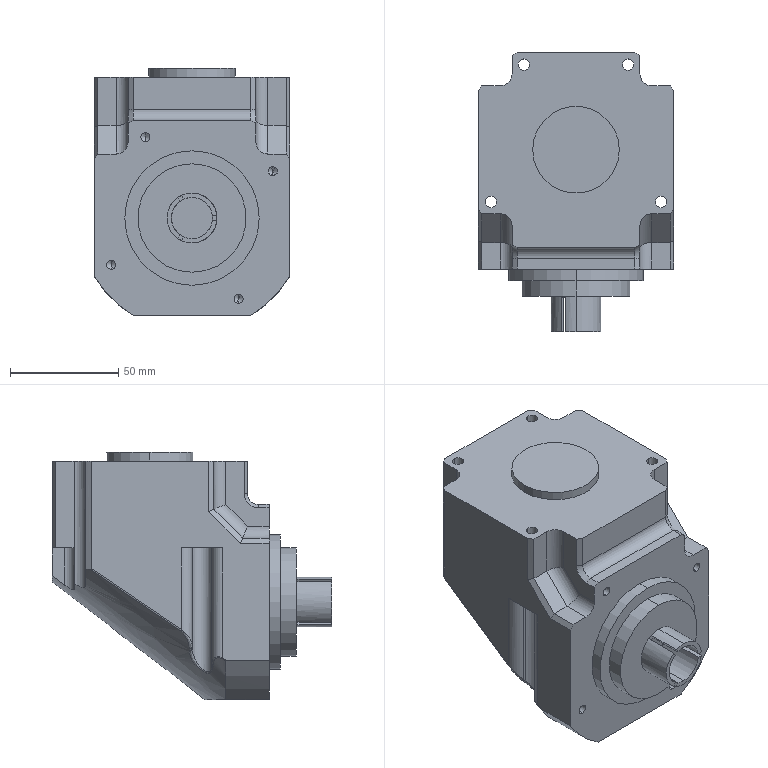Part | SolidWorks | features BaseBody 1 | 1 solid | 135 faces | box 90 x 128.8 x 114 mm | volume 723669 mm3 | cylinder 61 | plane 49 | spline 15 | cone 8 | torus 2 | commonest cylinder face diameters 105 x16 4.2 x8 5.3 x8 11 x8 10 x5 9 x4